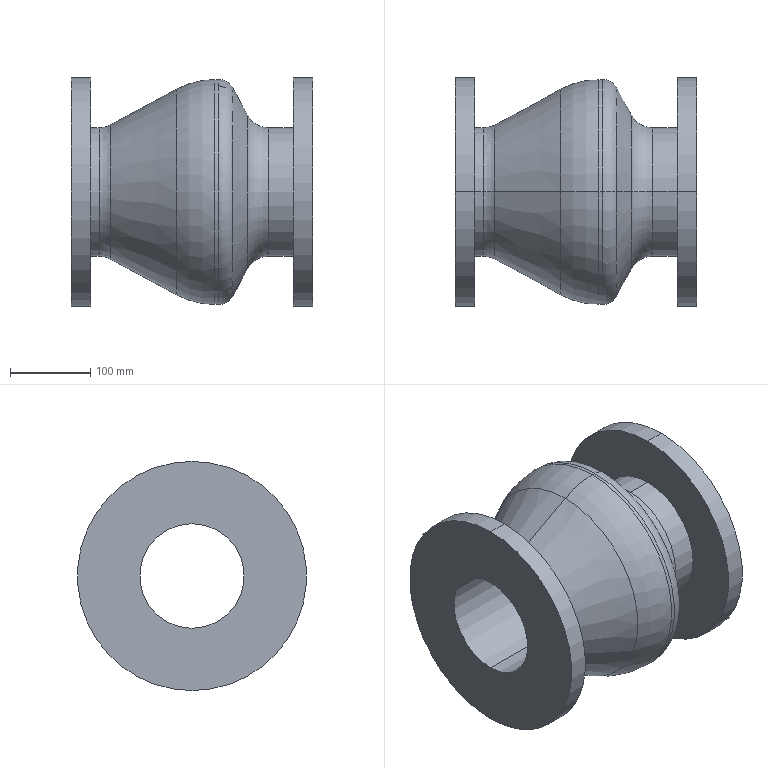Part | SolidWorks | features Revolution 1 | 1 solid | 28 faces | box 300 x 285 x 285 mm | volume 8540460 mm3 | cylinder 12 | torus 8 | cone 4 | plane 4 | commonest cylinder face diameters 160 x4 285 x4 130 x2 279.772 x2
STEP:
#1=CARTESIAN_POINT('',(34.398,0.,80.));
#2=VERTEX_POINT('',#1);
#3=CARTESIAN_POINT('',(34.398,0.,-80.));
#4=VERTEX_POINT('',#3);
#5=CARTESIAN_POINT('',(34.398,0.,0.));
#6=DIRECTION('',(-1.,0.,0.));
#7=DIRECTION('',(0.,0.,1.));
#8=AXIS2_PLACEMENT_3D('',#5,#6,#7);
#9=CIRCLE('',#8,80.);
#10=EDGE_CURVE('',#2,#4,#9,.T.);
#11=ORIENTED_EDGE('',*,*,#10,.T.);
#12=CARTESIAN_POINT('',(24.,0.,-80.));
#13=VERTEX_POINT('',#12);
#14=CARTESIAN_POINT('',(0.,0.,-80.));
#15=DIRECTION('',(-1.,0.,0.));
#16=VECTOR('',#15,1000.);
#17=LINE('',#14,#16);
#18=EDGE_CURVE('',#4,#13,#17,.T.);
#19=ORIENTED_EDGE('',*,*,#18,.T.);
#20=CARTESIAN_POINT('',(24.,0.,80.));
#21=VERTEX_POINT('',#20);
#22=CARTESIAN_POINT('',(24.,0.,0.));
#23=DIRECTION('',(-1.,0.,0.));
#24=DIRECTION('',(0.,0.,1.));
#25=AXIS2_PLACEMENT_3D('',#22,#23,#24);
#26=CIRCLE('',#25,80.);
#27=EDGE_CURVE('',#21,#13,#26,.T.);
#28=ORIENTED_EDGE('',*,*,#27,.F.);
#29=CARTESIAN_POINT('',(0.,0.,80.));
#30=DIRECTION('',(-1.,0.,0.));
#31=VECTOR('',#30,1000.);
#32=LINE('',#29,#31);
#33=EDGE_CURVE('',#2,#21,#32,.T.);
#34=ORIENTED_EDGE('',*,*,#33,.F.);
#35=EDGE_LOOP('',(#11,#19,#28,#34));
#36=FACE_OUTER_BOUND('',#35,.T.);
#37=CARTESIAN_POINT('',(0.,0.,0.));
#38=DIRECTION('',(-1.,0.,0.));
#39=DIRECTION('',(0.,0.,1.));
#40=AXIS2_PLACEMENT_3D('',#37,#38,#39);
#41=CYLINDRICAL_SURFACE('',#40,80.);
#42=ADVANCED_FACE('',(#36),#41,.T.);
#43=CARTESIAN_POINT('',(34.398,0.,0.));
#44=DIRECTION('',(-1.,0.,0.));
#45=DIRECTION('',(0.,0.,1.));
#46=AXIS2_PLACEMENT_3D('',#43,#44,#45);
#47=CIRCLE('',#46,80.);
#48=EDGE_CURVE('',#4,#2,#47,.T.);
#49=ORIENTED_EDGE('',*,*,#48,.F.);
#50=CARTESIAN_POINT('',(48.621,0.,-83.586));
#51=VERTEX_POINT('',#50);
#52=CARTESIAN_POINT('',(34.398,0.,-110.));
#53=DIRECTION('',(0.,1.,0.));
#54=DIRECTION('',(0.,0.,1.));
#55=AXIS2_PLACEMENT_3D('',#52,#53,#54);
#56=CIRCLE('',#55,30.);
#57=EDGE_CURVE('',#4,#51,#56,.T.);
#58=ORIENTED_EDGE('',*,*,#57,.T.);
#59=CARTESIAN_POINT('',(48.621,0.,83.586));
#60=VERTEX_POINT('',#59);
#61=CARTESIAN_POINT('',(48.621,0.,0.));
#62=DIRECTION('',(-1.,0.,0.));
#63=DIRECTION('',(0.,0.,1.));
#64=AXIS2_PLACEMENT_3D('',#61,#62,#63);
#65=CIRCLE('',#64,83.586);
#66=EDGE_CURVE('',#51,#60,#65,.T.);
#67=ORIENTED_EDGE('',*,*,#66,.T.);
#68=CARTESIAN_POINT('',(34.398,0.,110.));
#69=DIRECTION('',(0.,-1.,0.));
#70=DIRECTION('',(0.,0.,-1.));
#71=AXIS2_PLACEMENT_3D('',#68,#69,#70);
#72=CIRCLE('',#71,30.);
#73=EDGE_CURVE('',#2,#60,#72,.T.);
#74=ORIENTED_EDGE('',*,*,#73,.F.);
#75=EDGE_LOOP('',(#49,#58,#67,#74));
#76=FACE_OUTER_BOUND('',#75,.T.);
#77=CARTESIAN_POINT('',(34.398,0.,0.));
#78=DIRECTION('',(-1.,0.,0.));
#79=DIRECTION('',(0.,0.,1.));
#80=AXIS2_PLACEMENT_3D('',#77,#78,#79);
#81=TOROIDAL_SURFACE('',#80,110.,30.);
#82=ADVANCED_FACE('',(#76),#81,.F.);
#83=CARTESIAN_POINT('',(48.621,0.,0.));
#84=DIRECTION('',(-1.,0.,0.));
#85=DIRECTION('',(0.,0.,1.));
#86=AXIS2_PLACEMENT_3D('',#83,#84,#85);
#87=CIRCLE('',#86,83.586);
#88=EDGE_CURVE('',#60,#51,#87,.T.);
#89=ORIENTED_EDGE('',*,*,#88,.F.);
#90=CARTESIAN_POINT('',(130.98,0.,127.933));
#91=VERTEX_POINT('',#90);
#92=CARTESIAN_POINT('',(130.98,0.,127.933));
#93=DIRECTION('',(0.8805,0.,0.4741));
#94=VECTOR('',#93,1000.);
#95=LINE('',#92,#94);
#96=EDGE_CURVE('',#60,#91,#95,.T.);
#97=ORIENTED_EDGE('',*,*,#96,.T.);
#98=CARTESIAN_POINT('',(130.98,0.,-127.933));
#99=VERTEX_POINT('',#98);
#100=CARTESIAN_POINT('',(130.98,0.,0.));
#101=DIRECTION('',(-1.,0.,0.));
#102=DIRECTION('',(0.,0.,1.));
#103=AXIS2_PLACEMENT_3D('',#100,#101,#102);
#104=CIRCLE('',#103,127.933);
#105=EDGE_CURVE('',#91,#99,#104,.T.);
#106=ORIENTED_EDGE('',*,*,#105,.T.);
#107=CARTESIAN_POINT('',(130.98,0.,-127.933));
#108=DIRECTION('',(0.8805,0.,-0.4741));
#109=VECTOR('',#108,1000.);
#110=LINE('',#107,#109);
#111=EDGE_CURVE('',#51,#99,#110,.T.);
#112=ORIENTED_EDGE('',*,*,#111,.F.);
#113=EDGE_LOOP('',(#89,#97,#106,#112));
#114=FACE_OUTER_BOUND('',#113,.T.);
#115=CARTESIAN_POINT('',(130.98,0.,0.));
#116=DIRECTION('',(1.,0.,0.));
#117=DIRECTION('',(0.,0.,-1.));
#118=AXIS2_PLACEMENT_3D('',#115,#116,#117);
#119=CONICAL_SURFACE('',#118,127.933,0.4939);
#120=ADVANCED_FACE('',(#114),#119,.T.);
#121=CARTESIAN_POINT('',(178.39,0.,139.886));
#122=VERTEX_POINT('',#121);
#123=CARTESIAN_POINT('',(178.39,0.,-139.886));
#124=VERTEX_POINT('',#123);
#125=CARTESIAN_POINT('',(178.39,0.,0.));
#126=DIRECTION('',(-1.,0.,0.));
#127=DIRECTION('',(0.,0.,1.));
#128=AXIS2_PLACEMENT_3D('',#125,#126,#127);
#129=CIRCLE('',#128,139.886);
#130=EDGE_CURVE('',#122,#124,#129,.T.);
#131=ORIENTED_EDGE('',*,*,#130,.T.);
#132=CARTESIAN_POINT('',(178.39,0.,-39.886));
#133=DIRECTION('',(0.,1.,0.));
#134=DIRECTION('',(0.,0.,1.));
#135=AXIS2_PLACEMENT_3D('',#132,#133,#134);
#136=CIRCLE('',#135,100.);
#137=EDGE_CURVE('',#124,#99,#136,.T.);
#138=ORIENTED_EDGE('',*,*,#137,.T.);
#139=ORIENTED_EDGE('',*,*,#105,.F.);
#140=CARTESIAN_POINT('',(178.39,0.,39.886));
#141=DIRECTION('',(0.,-1.,0.));
#142=DIRECTION('',(0.,0.,-1.));
#143=AXIS2_PLACEMENT_3D('',#140,#141,#142);
#144=CIRCLE('',#143,100.);
#145=EDGE_CURVE('',#122,#91,#144,.T.);
#146=ORIENTED_EDGE('',*,*,#145,.F.);
#147=EDGE_LOOP('',(#131,#138,#139,#146));
#148=FACE_OUTER_BOUND('',#147,.T.);
#149=CARTESIAN_POINT('',(178.39,0.,0.));
#150=DIRECTION('',(-1.,0.,0.));
#151=DIRECTION('',(0.,0.,1.));
#152=AXIS2_PLACEMENT_3D('',#149,#150,#151);
#153=TOROIDAL_SURFACE('',#152,39.886,100.);
#154=ADVANCED_FACE('',(#148),#153,.T.);
#155=CARTESIAN_POINT('',(183.058,0.,139.886));
#156=VERTEX_POINT('',#155);
#157=CARTESIAN_POINT('',(183.058,0.,-139.886));
#158=VERTEX_POINT('',#157);
#159=CARTESIAN_POINT('',(183.058,0.,0.));
#160=DIRECTION('',(-1.,0.,0.));
#161=DIRECTION('',(0.,0.,1.));
#162=AXIS2_PLACEMENT_3D('',#159,#160,#161);
#163=CIRCLE('',#162,139.886);
#164=EDGE_CURVE('',#156,#158,#163,.T.);
#165=ORIENTED_EDGE('',*,*,#164,.T.);
#166=CARTESIAN_POINT('',(0.,0.,-139.886));
#167=DIRECTION('',(-1.,0.,0.));
#168=VECTOR('',#167,1000.);
#169=LINE('',#166,#168);
#170=EDGE_CURVE('',#158,#124,#169,.T.);
#171=ORIENTED_EDGE('',*,*,#170,.T.);
#172=ORIENTED_EDGE('',*,*,#130,.F.);
#173=CARTESIAN_POINT('',(0.,0.,139.886));
#174=DIRECTION('',(-1.,0.,0.));
#175=VECTOR('',#174,1000.);
#176=LINE('',#173,#175);
#177=EDGE_CURVE('',#156,#122,#176,.T.);
#178=ORIENTED_EDGE('',*,*,#177,.F.);
#179=EDGE_LOOP('',(#165,#171,#172,#178));
#180=FACE_OUTER_BOUND('',#179,.T.);
#181=CARTESIAN_POINT('',(0.,0.,0.));
#182=DIRECTION('',(-1.,0.,0.));
#183=DIRECTION('',(0.,0.,1.));
#184=AXIS2_PLACEMENT_3D('',#181,#182,#183);
#185=CYLINDRICAL_SURFACE('',#184,139.886);
#186=ADVANCED_FACE('',(#180),#185,.T.);
#187=CARTESIAN_POINT('',(200.667,0.,129.368));
#188=VERTEX_POINT('',#187);
#189=CARTESIAN_POINT('',(200.667,0.,-129.368));
#190=VERTEX_POINT('',#189);
#191=CARTESIAN_POINT('',(200.667,0.,0.));
#192=DIRECTION('',(-1.,0.,0.));
#193=DIRECTION('',(0.,0.,1.));
#194=AXIS2_PLACEMENT_3D('',#191,#192,#193);
#195=CIRCLE('',#194,129.368);
#196=EDGE_CURVE('',#188,#190,#195,.T.);
#197=ORIENTED_EDGE('',*,*,#196,.T.);
#198=CARTESIAN_POINT('',(183.058,0.,-119.886));
#199=DIRECTION('',(0.,1.,0.));
#200=DIRECTION('',(0.,0.,1.));
#201=AXIS2_PLACEMENT_3D('',#198,#199,#200);
#202=CIRCLE('',#201,20.);
#203=EDGE_CURVE('',#190,#158,#202,.T.);
#204=ORIENTED_EDGE('',*,*,#203,.T.);
#205=ORIENTED_EDGE('',*,*,#164,.F.);
#206=CARTESIAN_POINT('',(183.058,0.,119.886));
#207=DIRECTION('',(0.,-1.,0.));
#208=DIRECTION('',(0.,0.,-1.));
#209=AXIS2_PLACEMENT_3D('',#206,#207,#208);
#210=CIRCLE('',#209,20.);
#211=EDGE_CURVE('',#188,#156,#210,.T.);
#212=ORIENTED_EDGE('',*,*,#211,.F.);
#213=EDGE_LOOP('',(#197,#204,#205,#212));
#214=FACE_OUTER_BOUND('',#213,.T.);
#215=CARTESIAN_POINT('',(183.058,0.,0.));
#216=DIRECTION('',(-1.,0.,0.));
#217=DIRECTION('',(0.,0.,1.));
#218=AXIS2_PLACEMENT_3D('',#215,#216,#217);
#219=TOROIDAL_SURFACE('',#218,119.886,20.);
#220=ADVANCED_FACE('',(#214),#219,.T.);
#221=CARTESIAN_POINT('',(218.755,0.,95.777));
#222=VERTEX_POINT('',#221);
#223=CARTESIAN_POINT('',(218.755,0.,-95.777));
#224=VERTEX_POINT('',#223);
#225=CARTESIAN_POINT('',(218.755,0.,0.));
#226=DIRECTION('',(-1.,0.,0.));
#227=DIRECTION('',(0.,0.,1.));
#228=AXIS2_PLACEMENT_3D('',#225,#226,#227);
#229=CIRCLE('',#228,95.777);
#230=EDGE_CURVE('',#222,#224,#229,.T.);
#231=ORIENTED_EDGE('',*,*,#230,.T.);
#232=CARTESIAN_POINT('',(218.755,0.,-95.777));
#233=DIRECTION('',(-0.4741,0.,-0.8805));
#234=VECTOR('',#233,1000.);
#235=LINE('',#232,#234);
#236=EDGE_CURVE('',#224,#190,#235,.T.);
#237=ORIENTED_EDGE('',*,*,#236,.T.);
#238=ORIENTED_EDGE('',*,*,#196,.F.);
#239=CARTESIAN_POINT('',(218.755,0.,95.777));
#240=DIRECTION('',(-0.4741,0.,0.8805));
#241=VECTOR('',#240,1000.);
#242=LINE('',#239,#241);
#243=EDGE_CURVE('',#222,#188,#242,.T.);
#244=ORIENTED_EDGE('',*,*,#243,.F.);
#245=EDGE_LOOP('',(#231,#237,#238,#244));
#246=FACE_OUTER_BOUND('',#245,.T.);
#247=CARTESIAN_POINT('',(218.755,0.,0.));
#248=DIRECTION('',(-1.,0.,0.));
#249=DIRECTION('',(0.,0.,1.));
#250=AXIS2_PLACEMENT_3D('',#247,#248,#249);
#251=CONICAL_SURFACE('',#250,95.777,1.077);
#252=ADVANCED_FACE('',(#246),#251,.T.);
#253=CARTESIAN_POINT('',(218.755,0.,0.));
#254=DIRECTION('',(-1.,0.,0.));
#255=DIRECTION('',(0.,0.,1.));
#256=AXIS2_PLACEMENT_3D('',#253,#254,#255);
#257=CIRCLE('',#256,95.777);
#258=EDGE_CURVE('',#224,#222,#257,.T.);
#259=ORIENTED_EDGE('',*,*,#258,.F.);
#260=CARTESIAN_POINT('',(245.169,0.,-80.));
#261=VERTEX_POINT('',#260);
#262=CARTESIAN_POINT('',(245.169,0.,-110.));
#263=DIRECTION('',(0.,1.,0.));
#264=DIRECTION('',(0.,0.,1.));
#265=AXIS2_PLACEMENT_3D('',#262,#263,#264);
#266=CIRCLE('',#265,30.);
#267=EDGE_CURVE('',#224,#261,#266,.T.);
#268=ORIENTED_EDGE('',*,*,#267,.T.);
#269=CARTESIAN_POINT('',(245.169,0.,80.));
#270=VERTEX_POINT('',#269);
#271=CARTESIAN_POINT('',(245.169,0.,0.));
#272=DIRECTION('',(-1.,0.,0.));
#273=DIRECTION('',(0.,0.,1.));
#274=AXIS2_PLACEMENT_3D('',#271,#272,#273);
#275=CIRCLE('',#274,80.);
#276=EDGE_CURVE('',#261,#270,#275,.T.);
#277=ORIENTED_EDGE('',*,*,#276,.T.);
#278=CARTESIAN_POINT('',(245.169,0.,110.));
#279=DIRECTION('',(0.,-1.,0.));
#280=DIRECTION('',(0.,0.,-1.));
#281=AXIS2_PLACEMENT_3D('',#278,#279,#280);
#282=CIRCLE('',#281,30.);
#283=EDGE_CURVE('',#222,#270,#282,.T.);
#284=ORIENTED_EDGE('',*,*,#283,.F.);
#285=EDGE_LOOP('',(#259,#268,#277,#284));
#286=FACE_OUTER_BOUND('',#285,.T.);
#287=CARTESIAN_POINT('',(245.169,0.,0.));
#288=DIRECTION('',(-1.,0.,0.));
#289=DIRECTION('',(0.,0.,1.));
#290=AXIS2_PLACEMENT_3D('',#287,#288,#289);
#291=TOROIDAL_SURFACE('',#290,110.,30.);
#292=ADVANCED_FACE('',(#286),#291,.F.);
#293=CARTESIAN_POINT('',(276.,0.,80.));
#294=VERTEX_POINT('',#293);
#295=CARTESIAN_POINT('',(276.,0.,-80.));
#296=VERTEX_POINT('',#295);
#297=CARTESIAN_POINT('',(276.,0.,0.));
#298=DIRECTION('',(-1.,0.,0.));
#299=DIRECTION('',(0.,0.,1.));
#300=AXIS2_PLACEMENT_3D('',#297,#298,#299);
#301=CIRCLE('',#300,80.);
#302=EDGE_CURVE('',#294,#296,#301,.T.);
#303=ORIENTED_EDGE('',*,*,#302,.T.);
#304=CARTESIAN_POINT('',(0.,0.,-80.));
#305=DIRECTION('',(-1.,0.,0.));
#306=VECTOR('',#305,1000.);
#307=LINE('',#304,#306);
#308=EDGE_CURVE('',#296,#261,#307,.T.);
#309=ORIENTED_EDGE('',*,*,#308,.T.);
#310=CARTESIAN_POINT('',(245.169,0.,0.));
#311=DIRECTION('',(-1.,0.,0.));
#312=DIRECTION('',(0.,0.,1.));
#313=AXIS2_PLACEMENT_3D('',#310,#311,#312);
#314=CIRCLE('',#313,80.);
#315=EDGE_CURVE('',#270,#261,#314,.T.);
#316=ORIENTED_EDGE('',*,*,#315,.F.);
#317=CARTESIAN_POINT('',(0.,0.,80.));
#318=DIRECTION('',(-1.,0.,0.));
#319=VECTOR('',#318,1000.);
#320=LINE('',#317,#319);
#321=EDGE_CURVE('',#294,#270,#320,.T.);
#322=ORIENTED_EDGE('',*,*,#321,.F.);
#323=EDGE_LOOP('',(#303,#309,#316,#322));
#324=FACE_OUTER_BOUND('',#323,.T.);
#325=CARTESIAN_POINT('',(0.,0.,0.));
#326=DIRECTION('',(-1.,0.,0.));
#327=DIRECTION('',(0.,0.,1.));
#328=AXIS2_PLACEMENT_3D('',#325,#326,#327);
#329=CYLINDRICAL_SURFACE('',#328,80.);
#330=ADVANCED_FACE('',(#324),#329,.T.);
#331=CARTESIAN_POINT('',(300.,0.,142.5));
#332=VERTEX_POINT('',#331);
#333=CARTESIAN_POINT('',(300.,0.,-142.5));
#334=VERTEX_POINT('',#333);
#335=CARTESIAN_POINT('',(300.,0.,0.));
#336=DIRECTION('',(-1.,0.,0.));
#337=DIRECTION('',(0.,0.,1.));
#338=AXIS2_PLACEMENT_3D('',#335,#336,#337);
#339=CIRCLE('',#338,142.5);
#340=EDGE_CURVE('',#332,#334,#339,.T.);
#341=ORIENTED_EDGE('',*,*,#340,.T.);
#342=CARTESIAN_POINT('',(276.,0.,-142.5));
#343=VERTEX_POINT('',#342);
#344=CARTESIAN_POINT('',(0.,0.,-142.5));
#345=DIRECTION('',(-1.,0.,0.));
#346=VECTOR('',#345,1000.);
#347=LINE('',#344,#346);
#348=EDGE_CURVE('',#334,#343,#347,.T.);
#349=ORIENTED_EDGE('',*,*,#348,.T.);
#350=CARTESIAN_POINT('',(276.,0.,142.5));
#351=VERTEX_POINT('',#350);
#352=CARTESIAN_POINT('',(276.,0.,0.));
#353=DIRECTION('',(-1.,0.,0.));
#354=DIRECTION('',(0.,0.,1.));
#355=AXIS2_PLACEMENT_3D('',#352,#353,#354);
#356=CIRCLE('',#355,142.5);
#357=EDGE_CURVE('',#351,#343,#356,.T.);
#358=ORIENTED_EDGE('',*,*,#357,.F.);
#359=CARTESIAN_POINT('',(0.,0.,142.5));
#360=DIRECTION('',(-1.,0.,0.));
#361=VECTOR('',#360,1000.);
#362=LINE('',#359,#361);
#363=EDGE_CURVE('',#332,#351,#362,.T.);
#364=ORIENTED_EDGE('',*,*,#363,.F.);
#365=EDGE_LOOP('',(#341,#349,#358,#364));
#366=FACE_OUTER_BOUND('',#365,.T.);
#367=CARTESIAN_POINT('',(0.,0.,0.));
#368=DIRECTION('',(-1.,0.,0.));
#369=DIRECTION('',(0.,0.,1.));
#370=AXIS2_PLACEMENT_3D('',#367,#368,#369);
#371=CYLINDRICAL_SURFACE('',#370,142.5);
#372=ADVANCED_FACE('',(#366),#371,.T.);
#373=CARTESIAN_POINT('',(300.,0.,-65.));
#374=VERTEX_POINT('',#373);
#375=CARTESIAN_POINT('',(300.,0.,65.));
#376=VERTEX_POINT('',#375);
#377=CARTESIAN_POINT('',(300.,0.,0.));
#378=DIRECTION('',(-1.,0.,0.));
#379=DIRECTION('',(0.,0.,1.));
#380=AXIS2_PLACEMENT_3D('',#377,#378,#379);
#381=CIRCLE('',#380,65.);
#382=EDGE_CURVE('',#374,#376,#381,.T.);
#383=ORIENTED_EDGE('',*,*,#382,.F.);
#384=CARTESIAN_POINT('',(0.,0.,-65.));
#385=VERTEX_POINT('',#384);
#386=CARTESIAN_POINT('',(0.,0.,-65.));
#387=DIRECTION('',(-1.,0.,0.));
#388=VECTOR('',#387,1000.);
#389=LINE('',#386,#388);
#390=EDGE_CURVE('',#374,#385,#389,.T.);
#391=ORIENTED_EDGE('',*,*,#390,.T.);
#392=CARTESIAN_POINT('',(0.,0.,65.));
#393=VERTEX_POINT('',#392);
#394=CARTESIAN_POINT('',(0.,0.,0.));
#395=DIRECTION('',(-1.,0.,0.));
#396=DIRECTION('',(0.,0.,1.));
#397=AXIS2_PLACEMENT_3D('',#394,#395,#396);
#398=CIRCLE('',#397,65.);
#399=EDGE_CURVE('',#385,#393,#398,.T.);
#400=ORIENTED_EDGE('',*,*,#399,.T.);
#401=CARTESIAN_POINT('',(0.,0.,65.));
#402=DIRECTION('',(-1.,0.,0.));
#403=VECTOR('',#402,1000.);
#404=LINE('',#401,#403);
#405=EDGE_CURVE('',#376,#393,#404,.T.);
#406=ORIENTED_EDGE('',*,*,#405,.F.);
#407=EDGE_LOOP('',(#383,#391,#400,#406));
#408=FACE_OUTER_BOUND('',#407,.T.);
#409=CARTESIAN_POINT('',(0.,0.,0.));
#410=DIRECTION('',(-1.,0.,0.));
#411=DIRECTION('',(0.,0.,1.));
#412=AXIS2_PLACEMENT_3D('',#409,#410,#411);
#413=CYLINDRICAL_SURFACE('',#412,65.);
#414=ADVANCED_FACE('',(#408),#413,.F.);
#415=CARTESIAN_POINT('',(24.,0.,142.5));
#416=VERTEX_POINT('',#415);
#417=CARTESIAN_POINT('',(24.,0.,-142.5));
#418=VERTEX_POINT('',#417);
#419=CARTESIAN_POINT('',(24.,0.,0.));
#420=DIRECTION('',(-1.,0.,0.));
#421=DIRECTION('',(0.,0.,1.));
#422=AXIS2_PLACEMENT_3D('',#419,#420,#421);
#423=CIRCLE('',#422,142.5);
#424=EDGE_CURVE('',#416,#418,#423,.T.);
#425=ORIENTED_EDGE('',*,*,#424,.T.);
#426=CARTESIAN_POINT('',(0.,0.,-142.5));
#427=VERTEX_POINT('',#426);
#428=CARTESIAN_POINT('',(0.,0.,-142.5));
#429=DIRECTION('',(-1.,0.,0.));
#430=VECTOR('',#429,1000.);
#431=LINE('',#428,#430);
#432=EDGE_CURVE('',#418,#427,#431,.T.);
#433=ORIENTED_EDGE('',*,*,#432,.T.);
#434=CARTESIAN_POINT('',(0.,0.,142.5));
#435=VERTEX_POINT('',#434);
#436=CARTESIAN_POINT('',(0.,0.,0.));
#437=DIRECTION('',(-1.,0.,0.));
#438=DIRECTION('',(0.,0.,1.));
#439=AXIS2_PLACEMENT_3D('',#436,#437,#438);
#440=CIRCLE('',#439,142.5);
#441=EDGE_CURVE('',#435,#427,#440,.T.);
#442=ORIENTED_EDGE('',*,*,#441,.F.);
#443=CARTESIAN_POINT('',(0.,0.,142.5));
#444=DIRECTION('',(-1.,0.,0.));
#445=VECTOR('',#444,1000.);
#446=LINE('',#443,#445);
#447=EDGE_CURVE('',#416,#435,#446,.T.);
#448=ORIENTED_EDGE('',*,*,#447,.F.);
#449=EDGE_LOOP('',(#425,#433,#442,#448));
#450=FACE_OUTER_BOUND('',#449,.T.);
#451=CARTESIAN_POINT('',(0.,0.,0.));
#452=DIRECTION('',(-1.,0.,0.));
#453=DIRECTION('',(0.,0.,1.));
#454=AXIS2_PLACEMENT_3D('',#451,#452,#453);
#455=CYLINDRICAL_SURFACE('',#454,142.5);
#456=ADVANCED_FACE('',(#450),#455,.T.);
#457=ORIENTED_EDGE('',*,*,#432,.F.);
#458=CARTESIAN_POINT('',(24.,0.,0.));
#459=DIRECTION('',(-1.,0.,0.));
#460=DIRECTION('',(0.,0.,1.));
#461=AXIS2_PLACEMENT_3D('',#458,#459,#460);
#462=CIRCLE('',#461,142.5);
#463=EDGE_CURVE('',#418,#416,#462,.T.);
#464=ORIENTED_EDGE('',*,*,#463,.T.);
#465=ORIENTED_EDGE('',*,*,#447,.T.);
#466=CARTESIAN_POINT('',(0.,0.,0.));
#467=DIRECTION('',(-1.,0.,0.));
#468=DIRECTION('',(0.,0.,1.));
#469=AXIS2_PLACEMENT_3D('',#466,#467,#468);
#470=CIRCLE('',#469,142.5);
#471=EDGE_CURVE('',#427,#435,#470,.T.);
#472=ORIENTED_EDGE('',*,*,#471,.F.);
#473=EDGE_LOOP('',(#457,#464,#465,#472));
#474=FACE_OUTER_BOUND('',#473,.T.);
#475=CARTESIAN_POINT('',(0.,0.,0.));
#476=DIRECTION('',(-1.,0.,0.));
#477=DIRECTION('',(0.,0.,1.));
#478=AXIS2_PLACEMENT_3D('',#475,#476,#477);
#479=CYLINDRICAL_SURFACE('',#478,142.5);
#480=ADVANCED_FACE('',(#474),#479,.T.);
#481=CARTESIAN_POINT('',(0.,0.,0.));
#482=DIRECTION('',(-1.,0.,0.));
#483=DIRECTION('',(0.,0.,1.));
#484=AXIS2_PLACEMENT_3D('',#481,#482,#483);
#485=CIRCLE('',#484,65.);
#486=EDGE_CURVE('',#393,#385,#485,.T.);
#487=ORIENTED_EDGE('',*,*,#486,.F.);
#488=ORIENTED_EDGE('',*,*,#399,.F.);
#489=EDGE_LOOP('',(#487,#488));
#490=FACE_BOUND('',#489,.T.);
#491=ORIENTED_EDGE('',*,*,#441,.T.);
#492=ORIENTED_EDGE('',*,*,#471,.T.);
#493=EDGE_LOOP('',(#491,#492));
#494=FACE_OUTER_BOUND('',#493,.T.);
#495=CARTESIAN_POINT('',(0.,65.,0.));
#496=DIRECTION('',(1.,0.,0.));
#497=DIRECTION('',(0.,0.,-1.));
#498=AXIS2_PLACEMENT_3D('',#495,#496,#497);
#499=PLANE('',#498);
#500=ADVANCED_FACE('',(#490,#494),#499,.F.);
#501=ORIENTED_EDGE('',*,*,#390,.F.);
#502=CARTESIAN_POINT('',(300.,0.,0.));
#503=DIRECTION('',(-1.,0.,0.));
#504=DIRECTION('',(0.,0.,1.));
#505=AXIS2_PLACEMENT_3D('',#502,#503,#504);
#506=CIRCLE('',#505,65.);
#507=EDGE_CURVE('',#376,#374,#506,.T.);
#508=ORIENTED_EDGE('',*,*,#507,.F.);
#509=ORIENTED_EDGE('',*,*,#405,.T.);
#510=ORIENTED_EDGE('',*,*,#486,.T.);
#511=EDGE_LOOP('',(#501,#508,#509,#510));
#512=FACE_OUTER_BOUND('',#511,.T.);
#513=CARTESIAN_POINT('',(0.,0.,0.));
#514=DIRECTION('',(-1.,0.,0.));
#515=DIRECTION('',(0.,0.,1.));
#516=AXIS2_PLACEMENT_3D('',#513,#514,#515);
#517=CYLINDRICAL_SURFACE('',#516,65.);
#518=ADVANCED_FACE('',(#512),#517,.F.);
#519=ORIENTED_EDGE('',*,*,#340,.F.);
#520=CARTESIAN_POINT('',(300.,0.,0.));
#521=DIRECTION('',(-1.,0.,0.));
#522=DIRECTION('',(0.,0.,1.));
#523=AXIS2_PLACEMENT_3D('',#520,#521,#522);
#524=CIRCLE('',#523,142.5);
#525=EDGE_CURVE('',#334,#332,#524,.T.);
#526=ORIENTED_EDGE('',*,*,#525,.F.);
#527=EDGE_LOOP('',(#519,#526));
#528=FACE_OUTER_BOUND('',#527,.T.);
#529=ORIENTED_EDGE('',*,*,#507,.T.);
#530=ORIENTED_EDGE('',*,*,#382,.T.);
#531=EDGE_LOOP('',(#529,#530));
#532=FACE_BOUND('',#531,.T.);
#533=CARTESIAN_POINT('',(300.,142.5,0.));
#534=DIRECTION('',(-1.,0.,0.));
#535=DIRECTION('',(0.,0.,1.));
#536=AXIS2_PLACEMENT_3D('',#533,#534,#535);
#537=PLANE('',#536);
#538=ADVANCED_FACE('',(#528,#532),#537,.F.);
#539=ORIENTED_EDGE('',*,*,#348,.F.);
#540=ORIENTED_EDGE('',*,*,#525,.T.);
#541=ORIENTED_EDGE('',*,*,#363,.T.);
#542=CARTESIAN_POINT('',(276.,0.,0.));
#543=DIRECTION('',(-1.,0.,0.));
#544=DIRECTION('',(0.,0.,1.));
#545=AXIS2_PLACEMENT_3D('',#542,#543,#544);
#546=CIRCLE('',#545,142.5);
#547=EDGE_CURVE('',#343,#351,#546,.T.);
#548=ORIENTED_EDGE('',*,*,#547,.F.);
#549=EDGE_LOOP('',(#539,#540,#541,#548));
#550=FACE_OUTER_BOUND('',#549,.T.);
#551=CARTESIAN_POINT('',(0.,0.,0.));
#552=DIRECTION('',(-1.,0.,0.));
#553=DIRECTION('',(0.,0.,1.));
#554=AXIS2_PLACEMENT_3D('',#551,#552,#553);
#555=CYLINDRICAL_SURFACE('',#554,142.5);
#556=ADVANCED_FACE('',(#550),#555,.T.);
#557=ORIENTED_EDGE('',*,*,#302,.F.);
#558=CARTESIAN_POINT('',(276.,0.,0.));
#559=DIRECTION('',(-1.,0.,0.));
#560=DIRECTION('',(0.,0.,1.));
#561=AXIS2_PLACEMENT_3D('',#558,#559,#560);
#562=CIRCLE('',#561,80.);
#563=EDGE_CURVE('',#296,#294,#562,.T.);
#564=ORIENTED_EDGE('',*,*,#563,.F.);
#565=EDGE_LOOP('',(#557,#564));
#566=FACE_BOUND('',#565,.T.);
#567=ORIENTED_EDGE('',*,*,#357,.T.);
#568=ORIENTED_EDGE('',*,*,#547,.T.);
#569=EDGE_LOOP('',(#567,#568));
#570=FACE_OUTER_BOUND('',#569,.T.);
#571=CARTESIAN_POINT('',(276.,80.,0.));
#572=DIRECTION('',(1.,0.,0.));
#573=DIRECTION('',(0.,0.,-1.));
#574=AXIS2_PLACEMENT_3D('',#571,#572,#573);
#575=PLANE('',#574);
#576=ADVANCED_FACE('',(#566,#570),#575,.F.);
#577=ORIENTED_EDGE('',*,*,#308,.F.);
#578=ORIENTED_EDGE('',*,*,#563,.T.);
#579=ORIENTED_EDGE('',*,*,#321,.T.);
#580=ORIENTED_EDGE('',*,*,#276,.F.);
#581=EDGE_LOOP('',(#577,#578,#579,#580));
#582=FACE_OUTER_BOUND('',#581,.T.);
#583=CARTESIAN_POINT('',(0.,0.,0.));
#584=DIRECTION('',(-1.,0.,0.));
#585=DIRECTION('',(0.,0.,1.));
#586=AXIS2_PLACEMENT_3D('',#583,#584,#585);
#587=CYLINDRICAL_SURFACE('',#586,80.);
#588=ADVANCED_FACE('',(#582),#587,.T.);
#589=ORIENTED_EDGE('',*,*,#267,.F.);
#590=ORIENTED_EDGE('',*,*,#230,.F.);
#591=ORIENTED_EDGE('',*,*,#283,.T.);
#592=ORIENTED_EDGE('',*,*,#315,.T.);
#593=EDGE_LOOP('',(#589,#590,#591,#592));
#594=FACE_OUTER_BOUND('',#593,.T.);
#595=CARTESIAN_POINT('',(245.169,0.,0.));
#596=DIRECTION('',(-1.,0.,0.));
#597=DIRECTION('',(0.,0.,1.));
#598=AXIS2_PLACEMENT_3D('',#595,#596,#597);
#599=TOROIDAL_SURFACE('',#598,110.,30.);
#600=ADVANCED_FACE('',(#594),#599,.F.);
#601=ORIENTED_EDGE('',*,*,#236,.F.);
#602=ORIENTED_EDGE('',*,*,#258,.T.);
#603=ORIENTED_EDGE('',*,*,#243,.T.);
#604=CARTESIAN_POINT('',(200.667,0.,0.));
#605=DIRECTION('',(-1.,0.,0.));
#606=DIRECTION('',(0.,0.,1.));
#607=AXIS2_PLACEMENT_3D('',#604,#605,#606);
#608=CIRCLE('',#607,129.368);
#609=EDGE_CURVE('',#190,#188,#608,.T.);
#610=ORIENTED_EDGE('',*,*,#609,.F.);
#611=EDGE_LOOP('',(#601,#602,#603,#610));
#612=FACE_OUTER_BOUND('',#611,.T.);
#613=CARTESIAN_POINT('',(218.755,0.,0.));
#614=DIRECTION('',(-1.,0.,0.));
#615=DIRECTION('',(0.,0.,1.));
#616=AXIS2_PLACEMENT_3D('',#613,#614,#615);
#617=CONICAL_SURFACE('',#616,95.777,1.077);
#618=ADVANCED_FACE('',(#612),#617,.T.);
#619=ORIENTED_EDGE('',*,*,#203,.F.);
#620=ORIENTED_EDGE('',*,*,#609,.T.);
#621=ORIENTED_EDGE('',*,*,#211,.T.);
#622=CARTESIAN_POINT('',(183.058,0.,0.));
#623=DIRECTION('',(-1.,0.,0.));
#624=DIRECTION('',(0.,0.,1.));
#625=AXIS2_PLACEMENT_3D('',#622,#623,#624);
#626=CIRCLE('',#625,139.886);
#627=EDGE_CURVE('',#158,#156,#626,.T.);
#628=ORIENTED_EDGE('',*,*,#627,.F.);
#629=EDGE_LOOP('',(#619,#620,#621,#628));
#630=FACE_OUTER_BOUND('',#629,.T.);
#631=CARTESIAN_POINT('',(183.058,0.,0.));
#632=DIRECTION('',(-1.,0.,0.));
#633=DIRECTION('',(0.,0.,1.));
#634=AXIS2_PLACEMENT_3D('',#631,#632,#633);
#635=TOROIDAL_SURFACE('',#634,119.886,20.);
#636=ADVANCED_FACE('',(#630),#635,.T.);
#637=ORIENTED_EDGE('',*,*,#170,.F.);
#638=ORIENTED_EDGE('',*,*,#627,.T.);
#639=ORIENTED_EDGE('',*,*,#177,.T.);
#640=CARTESIAN_POINT('',(178.39,0.,0.));
#641=DIRECTION('',(-1.,0.,0.));
#642=DIRECTION('',(0.,0.,1.));
#643=AXIS2_PLACEMENT_3D('',#640,#641,#642);
#644=CIRCLE('',#643,139.886);
#645=EDGE_CURVE('',#124,#122,#644,.T.);
#646=ORIENTED_EDGE('',*,*,#645,.F.);
#647=EDGE_LOOP('',(#637,#638,#639,#646));
#648=FACE_OUTER_BOUND('',#647,.T.);
#649=CARTESIAN_POINT('',(0.,0.,0.));
#650=DIRECTION('',(-1.,0.,0.));
#651=DIRECTION('',(0.,0.,1.));
#652=AXIS2_PLACEMENT_3D('',#649,#650,#651);
#653=CYLINDRICAL_SURFACE('',#652,139.886);
#654=ADVANCED_FACE('',(#648),#653,.T.);
#655=ORIENTED_EDGE('',*,*,#137,.F.);
#656=ORIENTED_EDGE('',*,*,#645,.T.);
#657=ORIENTED_EDGE('',*,*,#145,.T.);
#658=CARTESIAN_POINT('',(130.98,0.,0.));
#659=DIRECTION('',(-1.,0.,0.));
#660=DIRECTION('',(0.,0.,1.));
#661=AXIS2_PLACEMENT_3D('',#658,#659,#660);
#662=CIRCLE('',#661,127.933);
#663=EDGE_CURVE('',#99,#91,#662,.T.);
#664=ORIENTED_EDGE('',*,*,#663,.F.);
#665=EDGE_LOOP('',(#655,#656,#657,#664));
#666=FACE_OUTER_BOUND('',#665,.T.);
#667=CARTESIAN_POINT('',(178.39,0.,0.));
#668=DIRECTION('',(-1.,0.,0.));
#669=DIRECTION('',(0.,0.,1.));
#670=AXIS2_PLACEMENT_3D('',#667,#668,#669);
#671=TOROIDAL_SURFACE('',#670,39.886,100.);
#672=ADVANCED_FACE('',(#666),#671,.T.);
#673=ORIENTED_EDGE('',*,*,#96,.F.);
#674=ORIENTED_EDGE('',*,*,#66,.F.);
#675=ORIENTED_EDGE('',*,*,#111,.T.);
#676=ORIENTED_EDGE('',*,*,#663,.T.);
#677=EDGE_LOOP('',(#673,#674,#675,#676));
#678=FACE_OUTER_BOUND('',#677,.T.);
#679=CARTESIAN_POINT('',(130.98,0.,0.));
#680=DIRECTION('',(1.,0.,0.));
#681=DIRECTION('',(0.,0.,-1.));
#682=AXIS2_PLACEMENT_3D('',#679,#680,#681);
#683=CONICAL_SURFACE('',#682,127.933,0.4939);
#684=ADVANCED_FACE('',(#678),#683,.T.);
#685=ORIENTED_EDGE('',*,*,#57,.F.);
#686=ORIENTED_EDGE('',*,*,#10,.F.);
#687=ORIENTED_EDGE('',*,*,#73,.T.);
#688=ORIENTED_EDGE('',*,*,#88,.T.);
#689=EDGE_LOOP('',(#685,#686,#687,#688));
#690=FACE_OUTER_BOUND('',#689,.T.);
#691=CARTESIAN_POINT('',(34.398,0.,0.));
#692=DIRECTION('',(-1.,0.,0.));
#693=DIRECTION('',(0.,0.,1.));
#694=AXIS2_PLACEMENT_3D('',#691,#692,#693);
#695=TOROIDAL_SURFACE('',#694,110.,30.);
#696=ADVANCED_FACE('',(#690),#695,.F.);
#697=ORIENTED_EDGE('',*,*,#18,.F.);
#698=ORIENTED_EDGE('',*,*,#48,.T.);
#699=ORIENTED_EDGE('',*,*,#33,.T.);
#700=CARTESIAN_POINT('',(24.,0.,0.));
#701=DIRECTION('',(-1.,0.,0.));
#702=DIRECTION('',(0.,0.,1.));
#703=AXIS2_PLACEMENT_3D('',#700,#701,#702);
#704=CIRCLE('',#703,80.);
#705=EDGE_CURVE('',#13,#21,#704,.T.);
#706=ORIENTED_EDGE('',*,*,#705,.F.);
#707=EDGE_LOOP('',(#697,#698,#699,#706));
#708=FACE_OUTER_BOUND('',#707,.T.);
#709=CARTESIAN_POINT('',(0.,0.,0.));
#710=DIRECTION('',(-1.,0.,0.));
#711=DIRECTION('',(0.,0.,1.));
#712=AXIS2_PLACEMENT_3D('',#709,#710,#711);
#713=CYLINDRICAL_SURFACE('',#712,80.);
#714=ADVANCED_FACE('',(#708),#713,.T.);
#715=ORIENTED_EDGE('',*,*,#424,.F.);
#716=ORIENTED_EDGE('',*,*,#463,.F.);
#717=EDGE_LOOP('',(#715,#716));
#718=FACE_OUTER_BOUND('',#717,.T.);
#719=ORIENTED_EDGE('',*,*,#27,.T.);
#720=ORIENTED_EDGE('',*,*,#705,.T.);
#721=EDGE_LOOP('',(#719,#720));
#722=FACE_BOUND('',#721,.T.);
#723=CARTESIAN_POINT('',(24.,142.5,0.));
#724=DIRECTION('',(-1.,0.,0.));
#725=DIRECTION('',(0.,0.,1.));
#726=AXIS2_PLACEMENT_3D('',#723,#724,#725);
#727=PLANE('',#726);
#728=ADVANCED_FACE('',(#718,#722),#727,.F.);
#729=CLOSED_SHELL('',(#42,#82,#120,#154,#186,#220,#252,#292,#330,#372,#414,#456,#480,#500,#518,#538,#556,#576,#588,#600,#618,#636,#654,#672,#684,#696,#714,#728));
#730=MANIFOLD_SOLID_BREP('',#729);
#731=CARTESIAN_POINT('',(0.,0.,0.));
#732=DIRECTION('',(0.,0.,1.));
#733=DIRECTION('',(1.,0.,0.));
#734=AXIS2_PLACEMENT_3D('',#731,#732,#733);
#735=(LENGTH_UNIT()NAMED_UNIT(*)SI_UNIT(.MILLI.,.METRE.));
#736=UNCERTAINTY_MEASURE_WITH_UNIT(LENGTH_MEASURE(0.00001),#735,'','');
#737=(NAMED_UNIT(*)PLANE_ANGLE_UNIT()SI_UNIT($,.RADIAN.));
#738=(NAMED_UNIT(*)SI_UNIT($,.STERADIAN.)SOLID_ANGLE_UNIT());
#739=(GEOMETRIC_REPRESENTATION_CONTEXT(3)GLOBAL_UNCERTAINTY_ASSIGNED_CONTEXT((#736))GLOBAL_UNIT_ASSIGNED_CONTEXT((#735,#737,#738))REPRESENTATION_CONTEXT('',''));
#740=ADVANCED_BREP_SHAPE_REPRESENTATION('',(#730,#734),#739);